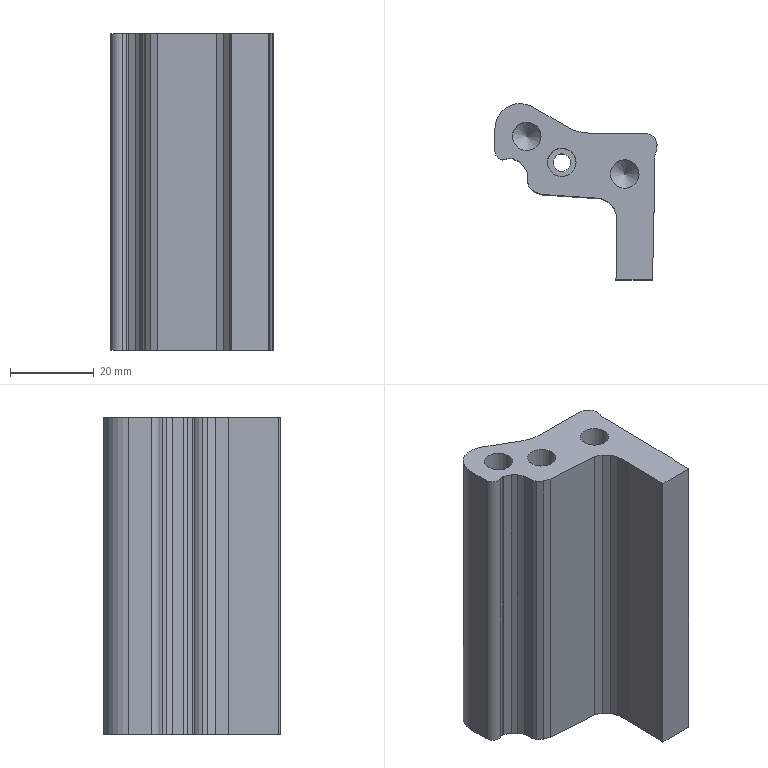Part | NX | features solid 2 | 1 solid | 40 faces | box 38.694 x 42.082 x 75.5 mm | volume 54302 mm3 | plane 26 | cylinder 11 | cone 3 | commonest cylinder face diameters 6.8 x3 4 x2 6 x2 4.2 x1 5.2 x1 12 x1
STEP:
#1=CARTESIAN_POINT('',(63.524,-37.821,-5.5));
#2=VERTEX_POINT('',#1);
#3=CARTESIAN_POINT('',(60.924,-37.821,-5.5));
#4=DIRECTION('',(0.,0.,1.));
#5=DIRECTION('',(1.,0.,0.));
#6=AXIS2_PLACEMENT_3D('',#3,#4,#5);
#7=CIRCLE('',#6,2.6);
#8=EDGE_CURVE('',#2,#2,#7,.T.);
#9=ORIENTED_EDGE('',*,*,#8,.T.);
#10=EDGE_LOOP('',(#9));
#11=FACE_BOUND('',#10,.T.);
#12=CARTESIAN_POINT('',(74.016,-60.221,-5.5));
#13=VERTEX_POINT('',#12);
#14=CARTESIAN_POINT('',(73.954,-65.044,-5.5));
#15=VERTEX_POINT('',#14);
#16=CARTESIAN_POINT('',(74.016,-60.221,-5.5));
#17=DIRECTION('',(-0.01273,-0.9999,0.));
#18=VECTOR('',#17,1000.);
#19=LINE('',#16,#18);
#20=EDGE_CURVE('',#13,#15,#19,.T.);
#21=ORIENTED_EDGE('',*,*,#20,.T.);
#22=CARTESIAN_POINT('',(65.247,-65.044,-5.5));
#23=VERTEX_POINT('',#22);
#24=CARTESIAN_POINT('',(40.003,-65.044,-5.5));
#25=DIRECTION('',(-1.,0.,0.));
#26=VECTOR('',#25,1000.);
#27=LINE('',#24,#26);
#28=EDGE_CURVE('',#15,#23,#27,.T.);
#29=ORIENTED_EDGE('',*,*,#28,.T.);
#30=CARTESIAN_POINT('',(65.303,-64.563,-5.5));
#31=VERTEX_POINT('',#30);
#32=CARTESIAN_POINT('',(63.441,-80.376,-5.5));
#33=DIRECTION('',(0.117,0.9931,0.));
#34=VECTOR('',#33,1000.);
#35=LINE('',#32,#34);
#36=EDGE_CURVE('',#23,#31,#35,.T.);
#37=ORIENTED_EDGE('',*,*,#36,.T.);
#38=CARTESIAN_POINT('',(65.509,-52.772,-5.5));
#39=VERTEX_POINT('',#38);
#40=CARTESIAN_POINT('',(65.303,-64.563,-5.5));
#41=DIRECTION('',(0.01745,0.9998,0.));
#42=VECTOR('',#41,1000.);
#43=LINE('',#40,#42);
#44=EDGE_CURVE('',#31,#39,#43,.T.);
#45=ORIENTED_EDGE('',*,*,#44,.T.);
#46=CARTESIAN_POINT('',(65.447,-49.66,-5.5));
#47=VERTEX_POINT('',#46);
#48=CARTESIAN_POINT('',(65.509,-52.772,-5.5));
#49=DIRECTION('',(-0.02008,0.9998,0.));
#50=VECTOR('',#49,1000.);
#51=LINE('',#48,#50);
#52=EDGE_CURVE('',#39,#47,#51,.T.);
#53=ORIENTED_EDGE('',*,*,#52,.T.);
#54=CARTESIAN_POINT('',(64.727,-47.823,-5.5));
#55=VERTEX_POINT('',#54);
#56=CARTESIAN_POINT('',(65.447,-49.66,-5.5));
#57=DIRECTION('',(-0.3648,0.9311,0.));
#58=VECTOR('',#57,1000.);
#59=LINE('',#56,#58);
#60=EDGE_CURVE('',#47,#55,#59,.T.);
#61=ORIENTED_EDGE('',*,*,#60,.T.);
#62=CARTESIAN_POINT('',(63.388,-46.401,-5.5));
#63=VERTEX_POINT('',#62);
#64=CARTESIAN_POINT('',(64.727,-47.823,-5.5));
#65=DIRECTION('',(-0.6854,0.7281,0.));
#66=VECTOR('',#65,1000.);
#67=LINE('',#64,#66);
#68=EDGE_CURVE('',#55,#63,#67,.T.);
#69=ORIENTED_EDGE('',*,*,#68,.T.);
#70=CARTESIAN_POINT('',(61.633,-45.601,-5.5));
#71=VERTEX_POINT('',#70);
#72=CARTESIAN_POINT('',(63.388,-46.401,-5.5));
#73=DIRECTION('',(-0.9101,0.4145,0.));
#74=VECTOR('',#73,1000.);
#75=LINE('',#72,#74);
#76=EDGE_CURVE('',#63,#71,#75,.T.);
#77=ORIENTED_EDGE('',*,*,#76,.T.);
#78=CARTESIAN_POINT('',(47.584,-44.653,-5.5));
#79=VERTEX_POINT('',#78);
#80=CARTESIAN_POINT('',(61.633,-45.601,-5.5));
#81=DIRECTION('',(-0.9977,0.06737,0.));
#82=VECTOR('',#81,1000.);
#83=LINE('',#80,#82);
#84=EDGE_CURVE('',#71,#79,#83,.T.);
#85=ORIENTED_EDGE('',*,*,#84,.T.);
#86=CARTESIAN_POINT('',(45.844,-44.031,-5.5));
#87=VERTEX_POINT('',#86);
#88=CARTESIAN_POINT('',(47.584,-44.653,-5.5));
#89=DIRECTION('',(-0.9417,0.3365,0.));
#90=VECTOR('',#89,1000.);
#91=LINE('',#88,#90);
#92=EDGE_CURVE('',#79,#87,#91,.T.);
#93=ORIENTED_EDGE('',*,*,#92,.T.);
#94=CARTESIAN_POINT('',(44.613,-42.954,-5.5));
#95=VERTEX_POINT('',#94);
#96=CARTESIAN_POINT('',(45.844,-44.031,-5.5));
#97=DIRECTION('',(-0.7529,0.6581,0.));
#98=VECTOR('',#97,1000.);
#99=LINE('',#96,#98);
#100=EDGE_CURVE('',#87,#95,#99,.T.);
#101=ORIENTED_EDGE('',*,*,#100,.T.);
#102=CARTESIAN_POINT('',(44.296,-42.082,-5.5));
#103=VERTEX_POINT('',#102);
#104=CARTESIAN_POINT('',(44.613,-42.954,-5.5));
#105=DIRECTION('',(-0.3407,0.9402,0.));
#106=VECTOR('',#105,1000.);
#107=LINE('',#104,#106);
#108=EDGE_CURVE('',#95,#103,#107,.T.);
#109=ORIENTED_EDGE('',*,*,#108,.T.);
#110=CARTESIAN_POINT('',(44.079,-39.402,-5.5));
#111=VERTEX_POINT('',#110);
#112=CARTESIAN_POINT('',(44.296,-42.082,-5.5));
#113=DIRECTION('',(-0.08071,0.9967,0.));
#114=VECTOR('',#113,1000.);
#115=LINE('',#112,#114);
#116=EDGE_CURVE('',#103,#111,#115,.T.);
#117=ORIENTED_EDGE('',*,*,#116,.T.);
#118=CARTESIAN_POINT('',(43.3,-37.914,-5.5));
#119=VERTEX_POINT('',#118);
#120=CARTESIAN_POINT('',(44.079,-39.402,-5.5));
#121=DIRECTION('',(-0.4639,0.8859,0.));
#122=VECTOR('',#121,1000.);
#123=LINE('',#120,#122);
#124=EDGE_CURVE('',#111,#119,#123,.T.);
#125=ORIENTED_EDGE('',*,*,#124,.T.);
#126=CARTESIAN_POINT('',(42.234,-36.887,-5.5));
#127=VERTEX_POINT('',#126);
#128=CARTESIAN_POINT('',(43.3,-37.914,-5.5));
#129=DIRECTION('',(-0.7204,0.6936,0.));
#130=VECTOR('',#129,1000.);
#131=LINE('',#128,#130);
#132=EDGE_CURVE('',#119,#127,#131,.T.);
#133=ORIENTED_EDGE('',*,*,#132,.T.);
#134=CARTESIAN_POINT('',(40.597,-36.034,-5.5));
#135=VERTEX_POINT('',#134);
#136=CARTESIAN_POINT('',(42.234,-36.887,-5.5));
#137=DIRECTION('',(-0.8867,0.4624,0.));
#138=VECTOR('',#137,1000.);
#139=LINE('',#136,#138);
#140=EDGE_CURVE('',#127,#135,#139,.T.);
#141=ORIENTED_EDGE('',*,*,#140,.T.);
#142=CARTESIAN_POINT('',(40.213,-35.993,-5.5));
#143=VERTEX_POINT('',#142);
#144=CARTESIAN_POINT('',(40.597,-36.034,-5.5));
#145=DIRECTION('',(-0.9945,0.105,0.));
#146=VECTOR('',#145,1000.);
#147=LINE('',#144,#146);
#148=EDGE_CURVE('',#135,#143,#147,.T.);
#149=ORIENTED_EDGE('',*,*,#148,.T.);
#150=CARTESIAN_POINT('',(39.206,-36.148,-5.5));
#151=VERTEX_POINT('',#150);
#152=CARTESIAN_POINT('',(40.003,-37.982,-5.5));
#153=DIRECTION('',(0.,0.,1.));
#154=DIRECTION('',(1.,0.,0.));
#155=AXIS2_PLACEMENT_3D('',#152,#153,#154);
#156=CIRCLE('',#155,2.);
#157=EDGE_CURVE('',#143,#151,#156,.T.);
#158=ORIENTED_EDGE('',*,*,#157,.T.);
#159=CARTESIAN_POINT('',(36.409,-34.313,-5.5));
#160=VERTEX_POINT('',#159);
#161=CARTESIAN_POINT('',(38.409,-34.313,-5.5));
#162=DIRECTION('',(0.,0.,-1.));
#163=DIRECTION('',(1.,0.,0.));
#164=AXIS2_PLACEMENT_3D('',#161,#162,#163);
#165=CIRCLE('',#164,2.);
#166=EDGE_CURVE('',#151,#160,#165,.T.);
#167=ORIENTED_EDGE('',*,*,#166,.T.);
#168=CARTESIAN_POINT('',(36.409,-28.962,-5.5));
#169=VERTEX_POINT('',#168);
#170=CARTESIAN_POINT('',(36.409,-34.313,-5.5));
#171=DIRECTION('',(0.,1.,0.));
#172=VECTOR('',#171,1000.);
#173=LINE('',#170,#172);
#174=EDGE_CURVE('',#160,#169,#173,.T.);
#175=ORIENTED_EDGE('',*,*,#174,.T.);
#176=CARTESIAN_POINT('',(45.409,-23.765,-5.5));
#177=VERTEX_POINT('',#176);
#178=CARTESIAN_POINT('',(42.409,-28.962,-5.5));
#179=DIRECTION('',(0.,0.,-1.));
#180=DIRECTION('',(1.,0.,0.));
#181=AXIS2_PLACEMENT_3D('',#178,#179,#180);
#182=CIRCLE('',#181,6.);
#183=EDGE_CURVE('',#169,#177,#182,.T.);
#184=ORIENTED_EDGE('',*,*,#183,.T.);
#185=CARTESIAN_POINT('',(53.924,-28.682,-5.5));
#186=VERTEX_POINT('',#185);
#187=CARTESIAN_POINT('',(45.409,-23.765,-5.5));
#188=DIRECTION('',(0.866,-0.5,0.));
#189=VECTOR('',#188,1000.);
#190=LINE('',#187,#189);
#191=EDGE_CURVE('',#177,#186,#190,.T.);
#192=ORIENTED_EDGE('',*,*,#191,.T.);
#193=CARTESIAN_POINT('',(58.924,-30.021,-5.5));
#194=VERTEX_POINT('',#193);
#195=CARTESIAN_POINT('',(58.924,-20.021,-5.5));
#196=DIRECTION('',(0.,0.,1.));
#197=DIRECTION('',(1.,0.,0.));
#198=AXIS2_PLACEMENT_3D('',#195,#196,#197);
#199=CIRCLE('',#198,10.);
#200=EDGE_CURVE('',#186,#194,#199,.T.);
#201=ORIENTED_EDGE('',*,*,#200,.T.);
#202=CARTESIAN_POINT('',(72.102,-30.021,-5.5));
#203=VERTEX_POINT('',#202);
#204=CARTESIAN_POINT('',(58.924,-30.021,-5.5));
#205=DIRECTION('',(1.,0.,0.));
#206=VECTOR('',#205,1000.);
#207=LINE('',#204,#206);
#208=EDGE_CURVE('',#194,#203,#207,.T.);
#209=ORIENTED_EDGE('',*,*,#208,.T.);
#210=CARTESIAN_POINT('',(74.849,-34.228,-5.5));
#211=VERTEX_POINT('',#210);
#212=CARTESIAN_POINT('',(72.102,-33.021,-5.5));
#213=DIRECTION('',(0.,0.,-1.));
#214=DIRECTION('',(1.,0.,0.));
#215=AXIS2_PLACEMENT_3D('',#212,#213,#214);
#216=CIRCLE('',#215,3.);
#217=EDGE_CURVE('',#203,#211,#216,.T.);
#218=ORIENTED_EDGE('',*,*,#217,.T.);
#219=CARTESIAN_POINT('',(74.596,-35.426,-5.5));
#220=VERTEX_POINT('',#219);
#221=CARTESIAN_POINT('',(77.596,-35.434,-5.5));
#222=DIRECTION('',(0.,0.,1.));
#223=DIRECTION('',(1.,0.,0.));
#224=AXIS2_PLACEMENT_3D('',#221,#222,#223);
#225=CIRCLE('',#224,3.);
#226=EDGE_CURVE('',#211,#220,#225,.T.);
#227=ORIENTED_EDGE('',*,*,#226,.T.);
#228=CARTESIAN_POINT('',(74.59,-37.317,-5.5));
#229=VERTEX_POINT('',#228);
#230=CARTESIAN_POINT('',(74.596,-35.426,-5.5));
#231=DIRECTION('',(-0.002751,-1.,0.));
#232=VECTOR('',#231,1000.);
#233=LINE('',#230,#232);
#234=EDGE_CURVE('',#220,#229,#233,.T.);
#235=ORIENTED_EDGE('',*,*,#234,.T.);
#236=CARTESIAN_POINT('',(74.168,-59.593,-5.5));
#237=VERTEX_POINT('',#236);
#238=CARTESIAN_POINT('',(74.59,-37.317,-5.5));
#239=DIRECTION('',(-0.01897,-0.9998,0.));
#240=VECTOR('',#239,1000.);
#241=LINE('',#238,#240);
#242=EDGE_CURVE('',#229,#237,#241,.T.);
#243=ORIENTED_EDGE('',*,*,#242,.T.);
#244=CARTESIAN_POINT('',(74.168,-59.593,-5.5));
#245=DIRECTION('',(-0.2353,-0.9719,0.));
#246=VECTOR('',#245,1000.);
#247=LINE('',#244,#246);
#248=EDGE_CURVE('',#237,#13,#247,.T.);
#249=ORIENTED_EDGE('',*,*,#248,.T.);
#250=EDGE_LOOP('',(#21,#29,#37,#45,#53,#61,#69,#77,#85,#93,#101,#109,#117,#125,#133,#141,#149,#158,#167,#175,#184,#192,#201,#209,#218,#227,#235,#243,#249));
#251=FACE_BOUND('',#250,.T.);
#252=CARTESIAN_POINT('',(54.463,-37.,-5.5));
#253=VERTEX_POINT('',#252);
#254=CARTESIAN_POINT('',(52.363,-37.,-5.5));
#255=DIRECTION('',(0.,0.,1.));
#256=DIRECTION('',(1.,0.,0.));
#257=AXIS2_PLACEMENT_3D('',#254,#255,#256);
#258=CIRCLE('',#257,2.1);
#259=EDGE_CURVE('',#253,#253,#258,.T.);
#260=ORIENTED_EDGE('',*,*,#259,.T.);
#261=EDGE_LOOP('',(#260));
#262=FACE_BOUND('',#261,.T.);
#263=CARTESIAN_POINT('',(40.003,-37.982,-5.5));
#264=DIRECTION('',(0.,0.,1.));
#265=DIRECTION('',(1.,0.,0.));
#266=AXIS2_PLACEMENT_3D('',#263,#264,#265);
#267=PLANE('',#266);
#268=ADVANCED_FACE('',(#11,#251,#262),#267,.F.);
#269=CARTESIAN_POINT('',(70.8,-39.8,70.));
#270=VERTEX_POINT('',#269);
#271=CARTESIAN_POINT('',(67.4,-39.8,70.));
#272=DIRECTION('',(0.,0.,-1.));
#273=DIRECTION('',(1.,0.,0.));
#274=AXIS2_PLACEMENT_3D('',#271,#272,#273);
#275=CIRCLE('',#274,3.4);
#276=EDGE_CURVE('',#270,#270,#275,.T.);
#277=ORIENTED_EDGE('',*,*,#276,.T.);
#278=EDGE_LOOP('',(#277));
#279=FACE_BOUND('',#278,.T.);
#280=CARTESIAN_POINT('',(73.954,-65.044,70.));
#281=VERTEX_POINT('',#280);
#282=CARTESIAN_POINT('',(65.247,-65.044,70.));
#283=VERTEX_POINT('',#282);
#284=CARTESIAN_POINT('',(-37.5,-65.044,70.));
#285=DIRECTION('',(-1.,0.,0.));
#286=VECTOR('',#285,1000.);
#287=LINE('',#284,#286);
#288=EDGE_CURVE('',#281,#283,#287,.T.);
#289=ORIENTED_EDGE('',*,*,#288,.F.);
#290=CARTESIAN_POINT('',(74.016,-60.221,70.));
#291=VERTEX_POINT('',#290);
#292=CARTESIAN_POINT('',(74.016,-60.221,70.));
#293=DIRECTION('',(-0.01273,-0.9999,0.));
#294=VECTOR('',#293,1000.);
#295=LINE('',#292,#294);
#296=EDGE_CURVE('',#291,#281,#295,.T.);
#297=ORIENTED_EDGE('',*,*,#296,.F.);
#298=CARTESIAN_POINT('',(74.168,-59.593,70.));
#299=VERTEX_POINT('',#298);
#300=CARTESIAN_POINT('',(74.168,-59.593,70.));
#301=DIRECTION('',(-0.2353,-0.9719,0.));
#302=VECTOR('',#301,1000.);
#303=LINE('',#300,#302);
#304=EDGE_CURVE('',#299,#291,#303,.T.);
#305=ORIENTED_EDGE('',*,*,#304,.F.);
#306=CARTESIAN_POINT('',(74.59,-37.317,70.));
#307=VERTEX_POINT('',#306);
#308=CARTESIAN_POINT('',(74.59,-37.317,70.));
#309=DIRECTION('',(-0.01897,-0.9998,0.));
#310=VECTOR('',#309,1000.);
#311=LINE('',#308,#310);
#312=EDGE_CURVE('',#307,#299,#311,.T.);
#313=ORIENTED_EDGE('',*,*,#312,.F.);
#314=CARTESIAN_POINT('',(74.596,-35.426,70.));
#315=VERTEX_POINT('',#314);
#316=CARTESIAN_POINT('',(74.596,-35.426,70.));
#317=DIRECTION('',(-0.002751,-1.,0.));
#318=VECTOR('',#317,1000.);
#319=LINE('',#316,#318);
#320=EDGE_CURVE('',#315,#307,#319,.T.);
#321=ORIENTED_EDGE('',*,*,#320,.F.);
#322=CARTESIAN_POINT('',(74.849,-34.228,70.));
#323=VERTEX_POINT('',#322);
#324=CARTESIAN_POINT('',(77.596,-35.434,70.));
#325=DIRECTION('',(0.,0.,1.));
#326=DIRECTION('',(1.,0.,0.));
#327=AXIS2_PLACEMENT_3D('',#324,#325,#326);
#328=CIRCLE('',#327,3.);
#329=EDGE_CURVE('',#323,#315,#328,.T.);
#330=ORIENTED_EDGE('',*,*,#329,.F.);
#331=CARTESIAN_POINT('',(72.102,-30.021,70.));
#332=VERTEX_POINT('',#331);
#333=CARTESIAN_POINT('',(72.102,-33.021,70.));
#334=DIRECTION('',(0.,0.,1.));
#335=DIRECTION('',(1.,0.,0.));
#336=AXIS2_PLACEMENT_3D('',#333,#334,#335);
#337=CIRCLE('',#336,3.);
#338=EDGE_CURVE('',#332,#323,#337,.F.);
#339=ORIENTED_EDGE('',*,*,#338,.F.);
#340=CARTESIAN_POINT('',(58.924,-30.021,70.));
#341=VERTEX_POINT('',#340);
#342=CARTESIAN_POINT('',(58.924,-30.021,70.));
#343=DIRECTION('',(1.,0.,0.));
#344=VECTOR('',#343,1000.);
#345=LINE('',#342,#344);
#346=EDGE_CURVE('',#341,#332,#345,.T.);
#347=ORIENTED_EDGE('',*,*,#346,.F.);
#348=CARTESIAN_POINT('',(53.924,-28.682,70.));
#349=VERTEX_POINT('',#348);
#350=CARTESIAN_POINT('',(58.924,-20.021,70.));
#351=DIRECTION('',(0.,0.,1.));
#352=DIRECTION('',(1.,0.,0.));
#353=AXIS2_PLACEMENT_3D('',#350,#351,#352);
#354=CIRCLE('',#353,10.);
#355=EDGE_CURVE('',#349,#341,#354,.T.);
#356=ORIENTED_EDGE('',*,*,#355,.F.);
#357=CARTESIAN_POINT('',(45.409,-23.765,70.));
#358=VERTEX_POINT('',#357);
#359=CARTESIAN_POINT('',(45.409,-23.765,70.));
#360=DIRECTION('',(0.866,-0.5,0.));
#361=VECTOR('',#360,1000.);
#362=LINE('',#359,#361);
#363=EDGE_CURVE('',#358,#349,#362,.T.);
#364=ORIENTED_EDGE('',*,*,#363,.F.);
#365=CARTESIAN_POINT('',(36.409,-28.962,70.));
#366=VERTEX_POINT('',#365);
#367=CARTESIAN_POINT('',(42.409,-28.962,70.));
#368=DIRECTION('',(0.,0.,1.));
#369=DIRECTION('',(1.,0.,0.));
#370=AXIS2_PLACEMENT_3D('',#367,#368,#369);
#371=CIRCLE('',#370,6.);
#372=EDGE_CURVE('',#366,#358,#371,.F.);
#373=ORIENTED_EDGE('',*,*,#372,.F.);
#374=CARTESIAN_POINT('',(36.409,-34.313,70.));
#375=VERTEX_POINT('',#374);
#376=CARTESIAN_POINT('',(36.409,-34.313,70.));
#377=DIRECTION('',(0.,1.,0.));
#378=VECTOR('',#377,1000.);
#379=LINE('',#376,#378);
#380=EDGE_CURVE('',#375,#366,#379,.T.);
#381=ORIENTED_EDGE('',*,*,#380,.F.);
#382=CARTESIAN_POINT('',(39.206,-36.148,70.));
#383=VERTEX_POINT('',#382);
#384=CARTESIAN_POINT('',(38.409,-34.313,70.));
#385=DIRECTION('',(0.,0.,1.));
#386=DIRECTION('',(1.,0.,0.));
#387=AXIS2_PLACEMENT_3D('',#384,#385,#386);
#388=CIRCLE('',#387,2.);
#389=EDGE_CURVE('',#383,#375,#388,.F.);
#390=ORIENTED_EDGE('',*,*,#389,.F.);
#391=CARTESIAN_POINT('',(40.213,-35.993,70.));
#392=VERTEX_POINT('',#391);
#393=CARTESIAN_POINT('',(40.003,-37.982,70.));
#394=DIRECTION('',(0.,0.,1.));
#395=DIRECTION('',(1.,0.,0.));
#396=AXIS2_PLACEMENT_3D('',#393,#394,#395);
#397=CIRCLE('',#396,2.);
#398=EDGE_CURVE('',#392,#383,#397,.T.);
#399=ORIENTED_EDGE('',*,*,#398,.F.);
#400=CARTESIAN_POINT('',(40.597,-36.034,70.));
#401=VERTEX_POINT('',#400);
#402=CARTESIAN_POINT('',(40.597,-36.034,70.));
#403=DIRECTION('',(-0.9945,0.105,0.));
#404=VECTOR('',#403,1000.);
#405=LINE('',#402,#404);
#406=EDGE_CURVE('',#401,#392,#405,.T.);
#407=ORIENTED_EDGE('',*,*,#406,.F.);
#408=CARTESIAN_POINT('',(42.234,-36.887,70.));
#409=VERTEX_POINT('',#408);
#410=CARTESIAN_POINT('',(42.234,-36.887,70.));
#411=DIRECTION('',(-0.8867,0.4624,0.));
#412=VECTOR('',#411,1000.);
#413=LINE('',#410,#412);
#414=EDGE_CURVE('',#409,#401,#413,.T.);
#415=ORIENTED_EDGE('',*,*,#414,.F.);
#416=CARTESIAN_POINT('',(43.3,-37.914,70.));
#417=VERTEX_POINT('',#416);
#418=CARTESIAN_POINT('',(43.3,-37.914,70.));
#419=DIRECTION('',(-0.7204,0.6936,0.));
#420=VECTOR('',#419,1000.);
#421=LINE('',#418,#420);
#422=EDGE_CURVE('',#417,#409,#421,.T.);
#423=ORIENTED_EDGE('',*,*,#422,.F.);
#424=CARTESIAN_POINT('',(44.079,-39.402,70.));
#425=VERTEX_POINT('',#424);
#426=CARTESIAN_POINT('',(44.079,-39.402,70.));
#427=DIRECTION('',(-0.4639,0.8859,0.));
#428=VECTOR('',#427,1000.);
#429=LINE('',#426,#428);
#430=EDGE_CURVE('',#425,#417,#429,.T.);
#431=ORIENTED_EDGE('',*,*,#430,.F.);
#432=CARTESIAN_POINT('',(44.296,-42.082,70.));
#433=VERTEX_POINT('',#432);
#434=CARTESIAN_POINT('',(44.296,-42.082,70.));
#435=DIRECTION('',(-0.08071,0.9967,0.));
#436=VECTOR('',#435,1000.);
#437=LINE('',#434,#436);
#438=EDGE_CURVE('',#433,#425,#437,.T.);
#439=ORIENTED_EDGE('',*,*,#438,.F.);
#440=CARTESIAN_POINT('',(44.613,-42.954,70.));
#441=VERTEX_POINT('',#440);
#442=CARTESIAN_POINT('',(44.613,-42.954,70.));
#443=DIRECTION('',(-0.3407,0.9402,0.));
#444=VECTOR('',#443,1000.);
#445=LINE('',#442,#444);
#446=EDGE_CURVE('',#441,#433,#445,.T.);
#447=ORIENTED_EDGE('',*,*,#446,.F.);
#448=CARTESIAN_POINT('',(45.844,-44.031,70.));
#449=VERTEX_POINT('',#448);
#450=CARTESIAN_POINT('',(45.844,-44.031,70.));
#451=DIRECTION('',(-0.7529,0.6581,0.));
#452=VECTOR('',#451,1000.);
#453=LINE('',#450,#452);
#454=EDGE_CURVE('',#441,#449,#453,.F.);
#455=ORIENTED_EDGE('',*,*,#454,.T.);
#456=CARTESIAN_POINT('',(47.584,-44.653,70.));
#457=VERTEX_POINT('',#456);
#458=CARTESIAN_POINT('',(47.584,-44.653,70.));
#459=DIRECTION('',(-0.9417,0.3365,0.));
#460=VECTOR('',#459,1000.);
#461=LINE('',#458,#460);
#462=EDGE_CURVE('',#449,#457,#461,.F.);
#463=ORIENTED_EDGE('',*,*,#462,.T.);
#464=CARTESIAN_POINT('',(61.633,-45.601,70.));
#465=VERTEX_POINT('',#464);
#466=CARTESIAN_POINT('',(61.633,-45.601,70.));
#467=DIRECTION('',(-0.9977,0.06737,0.));
#468=VECTOR('',#467,1000.);
#469=LINE('',#466,#468);
#470=EDGE_CURVE('',#457,#465,#469,.F.);
#471=ORIENTED_EDGE('',*,*,#470,.T.);
#472=CARTESIAN_POINT('',(63.388,-46.401,70.));
#473=VERTEX_POINT('',#472);
#474=CARTESIAN_POINT('',(63.388,-46.401,70.));
#475=DIRECTION('',(-0.9101,0.4145,0.));
#476=VECTOR('',#475,1000.);
#477=LINE('',#474,#476);
#478=EDGE_CURVE('',#465,#473,#477,.F.);
#479=ORIENTED_EDGE('',*,*,#478,.T.);
#480=CARTESIAN_POINT('',(64.727,-47.823,70.));
#481=VERTEX_POINT('',#480);
#482=CARTESIAN_POINT('',(64.727,-47.823,70.));
#483=DIRECTION('',(-0.6854,0.7281,0.));
#484=VECTOR('',#483,1000.);
#485=LINE('',#482,#484);
#486=EDGE_CURVE('',#473,#481,#485,.F.);
#487=ORIENTED_EDGE('',*,*,#486,.T.);
#488=CARTESIAN_POINT('',(65.447,-49.66,70.));
#489=VERTEX_POINT('',#488);
#490=CARTESIAN_POINT('',(65.447,-49.66,70.));
#491=DIRECTION('',(-0.3648,0.9311,0.));
#492=VECTOR('',#491,1000.);
#493=LINE('',#490,#492);
#494=EDGE_CURVE('',#481,#489,#493,.F.);
#495=ORIENTED_EDGE('',*,*,#494,.T.);
#496=CARTESIAN_POINT('',(65.509,-52.772,70.));
#497=VERTEX_POINT('',#496);
#498=CARTESIAN_POINT('',(65.509,-52.772,70.));
#499=DIRECTION('',(-0.02008,0.9998,0.));
#500=VECTOR('',#499,1000.);
#501=LINE('',#498,#500);
#502=EDGE_CURVE('',#489,#497,#501,.F.);
#503=ORIENTED_EDGE('',*,*,#502,.T.);
#504=CARTESIAN_POINT('',(65.303,-64.563,70.));
#505=VERTEX_POINT('',#504);
#506=CARTESIAN_POINT('',(65.303,-64.563,70.));
#507=DIRECTION('',(0.01745,0.9998,0.));
#508=VECTOR('',#507,1000.);
#509=LINE('',#506,#508);
#510=EDGE_CURVE('',#497,#505,#509,.F.);
#511=ORIENTED_EDGE('',*,*,#510,.T.);
#512=CARTESIAN_POINT('',(63.441,-80.376,70.));
#513=DIRECTION('',(0.117,0.9931,0.));
#514=VECTOR('',#513,1000.);
#515=LINE('',#512,#514);
#516=EDGE_CURVE('',#505,#283,#515,.F.);
#517=ORIENTED_EDGE('',*,*,#516,.T.);
#518=EDGE_LOOP('',(#289,#297,#305,#313,#321,#330,#339,#347,#356,#364,#373,#381,#390,#399,#407,#415,#423,#431,#439,#447,#455,#463,#471,#479,#487,#495,#503,#511,#517));
#519=FACE_BOUND('',#518,.T.);
#520=CARTESIAN_POINT('',(55.763,-37.,70.));
#521=VERTEX_POINT('',#520);
#522=CARTESIAN_POINT('',(52.363,-37.,70.));
#523=DIRECTION('',(0.,0.,1.));
#524=DIRECTION('',(1.,0.,0.));
#525=AXIS2_PLACEMENT_3D('',#522,#523,#524);
#526=CIRCLE('',#525,3.4);
#527=EDGE_CURVE('',#521,#521,#526,.T.);
#528=ORIENTED_EDGE('',*,*,#527,.F.);
#529=EDGE_LOOP('',(#528));
#530=FACE_BOUND('',#529,.T.);
#531=CARTESIAN_POINT('',(47.4,-30.8,70.));
#532=VERTEX_POINT('',#531);
#533=CARTESIAN_POINT('',(44.,-30.8,70.));
#534=DIRECTION('',(0.,0.,-1.));
#535=DIRECTION('',(1.,0.,0.));
#536=AXIS2_PLACEMENT_3D('',#533,#534,#535);
#537=CIRCLE('',#536,3.4);
#538=EDGE_CURVE('',#532,#532,#537,.T.);
#539=ORIENTED_EDGE('',*,*,#538,.T.);
#540=EDGE_LOOP('',(#539));
#541=FACE_BOUND('',#540,.T.);
#542=CARTESIAN_POINT('',(-37.5,0.,70.));
#543=DIRECTION('',(0.,0.,1.));
#544=DIRECTION('',(1.,0.,0.));
#545=AXIS2_PLACEMENT_3D('',#542,#543,#544);
#546=PLANE('',#545);
#547=ADVANCED_FACE('',(#279,#519,#530,#541),#546,.T.);
#548=ORIENTED_EDGE('',*,*,#510,.F.);
#549=CARTESIAN_POINT('',(65.509,-52.772,40.));
#550=DIRECTION('',(0.,0.,-1.));
#551=VECTOR('',#550,1000.);
#552=LINE('',#549,#551);
#553=EDGE_CURVE('',#497,#39,#552,.T.);
#554=ORIENTED_EDGE('',*,*,#553,.T.);
#555=ORIENTED_EDGE('',*,*,#44,.F.);
#556=CARTESIAN_POINT('',(65.303,-64.563,40.));
#557=DIRECTION('',(0.,0.,-1.));
#558=VECTOR('',#557,1000.);
#559=LINE('',#556,#558);
#560=EDGE_CURVE('',#505,#31,#559,.T.);
#561=ORIENTED_EDGE('',*,*,#560,.F.);
#562=EDGE_LOOP('',(#548,#554,#555,#561));
#563=FACE_BOUND('',#562,.T.);
#564=CARTESIAN_POINT('',(65.303,-64.563,40.));
#565=DIRECTION('',(-0.9998,0.01745,0.));
#566=DIRECTION('',(-0.01745,-0.9998,0.));
#567=AXIS2_PLACEMENT_3D('',#564,#565,#566);
#568=PLANE('',#567);
#569=ADVANCED_FACE('',(#563),#568,.T.);
#570=CARTESIAN_POINT('',(65.247,-65.044,40.));
#571=DIRECTION('',(0.,0.,-1.));
#572=VECTOR('',#571,1000.);
#573=LINE('',#570,#572);
#574=EDGE_CURVE('',#23,#283,#573,.F.);
#575=ORIENTED_EDGE('',*,*,#574,.T.);
#576=ORIENTED_EDGE('',*,*,#516,.F.);
#577=ORIENTED_EDGE('',*,*,#560,.T.);
#578=ORIENTED_EDGE('',*,*,#36,.F.);
#579=EDGE_LOOP('',(#575,#576,#577,#578));
#580=FACE_BOUND('',#579,.T.);
#581=CARTESIAN_POINT('',(63.441,-80.376,40.));
#582=DIRECTION('',(-0.9931,0.117,0.));
#583=DIRECTION('',(-0.117,-0.9931,0.));
#584=AXIS2_PLACEMENT_3D('',#581,#582,#583);
#585=PLANE('',#584);
#586=ADVANCED_FACE('',(#580),#585,.T.);
#587=CARTESIAN_POINT('',(73.954,-65.044,40.));
#588=DIRECTION('',(0.,0.,1.));
#589=VECTOR('',#588,1000.);
#590=LINE('',#587,#589);
#591=EDGE_CURVE('',#15,#281,#590,.T.);
#592=ORIENTED_EDGE('',*,*,#591,.F.);
#593=ORIENTED_EDGE('',*,*,#20,.F.);
#594=CARTESIAN_POINT('',(74.016,-60.221,40.));
#595=DIRECTION('',(0.,0.,-1.));
#596=VECTOR('',#595,1000.);
#597=LINE('',#594,#596);
#598=EDGE_CURVE('',#291,#13,#597,.T.);
#599=ORIENTED_EDGE('',*,*,#598,.F.);
#600=ORIENTED_EDGE('',*,*,#296,.T.);
#601=EDGE_LOOP('',(#592,#593,#599,#600));
#602=FACE_BOUND('',#601,.T.);
#603=CARTESIAN_POINT('',(74.016,-60.221,40.));
#604=DIRECTION('',(0.9999,-0.01273,0.));
#605=DIRECTION('',(0.01273,0.9999,0.));
#606=AXIS2_PLACEMENT_3D('',#603,#604,#605);
#607=PLANE('',#606);
#608=ADVANCED_FACE('',(#602),#607,.T.);
#609=CARTESIAN_POINT('',(74.168,-59.593,40.));
#610=DIRECTION('',(0.,0.,-1.));
#611=VECTOR('',#610,1000.);
#612=LINE('',#609,#611);
#613=EDGE_CURVE('',#299,#237,#612,.T.);
#614=ORIENTED_EDGE('',*,*,#613,.F.);
#615=ORIENTED_EDGE('',*,*,#304,.T.);
#616=ORIENTED_EDGE('',*,*,#598,.T.);
#617=ORIENTED_EDGE('',*,*,#248,.F.);
#618=EDGE_LOOP('',(#614,#615,#616,#617));
#619=FACE_BOUND('',#618,.T.);
#620=CARTESIAN_POINT('',(74.168,-59.593,40.));
#621=DIRECTION('',(0.9719,-0.2353,0.));
#622=DIRECTION('',(0.2353,0.9719,0.));
#623=AXIS2_PLACEMENT_3D('',#620,#621,#622);
#624=PLANE('',#623);
#625=ADVANCED_FACE('',(#619),#624,.T.);
#626=CARTESIAN_POINT('',(74.59,-37.317,40.));
#627=DIRECTION('',(0.,0.,-1.));
#628=VECTOR('',#627,1000.);
#629=LINE('',#626,#628);
#630=EDGE_CURVE('',#307,#229,#629,.T.);
#631=ORIENTED_EDGE('',*,*,#630,.F.);
#632=ORIENTED_EDGE('',*,*,#312,.T.);
#633=ORIENTED_EDGE('',*,*,#613,.T.);
#634=ORIENTED_EDGE('',*,*,#242,.F.);
#635=EDGE_LOOP('',(#631,#632,#633,#634));
#636=FACE_BOUND('',#635,.T.);
#637=CARTESIAN_POINT('',(74.59,-37.317,40.));
#638=DIRECTION('',(0.9998,-0.01897,0.));
#639=DIRECTION('',(0.01897,0.9998,0.));
#640=AXIS2_PLACEMENT_3D('',#637,#638,#639);
#641=PLANE('',#640);
#642=ADVANCED_FACE('',(#636),#641,.T.);
#643=CARTESIAN_POINT('',(74.596,-35.426,40.));
#644=DIRECTION('',(0.,0.,-1.));
#645=VECTOR('',#644,1000.);
#646=LINE('',#643,#645);
#647=EDGE_CURVE('',#315,#220,#646,.T.);
#648=ORIENTED_EDGE('',*,*,#647,.F.);
#649=ORIENTED_EDGE('',*,*,#320,.T.);
#650=ORIENTED_EDGE('',*,*,#630,.T.);
#651=ORIENTED_EDGE('',*,*,#234,.F.);
#652=EDGE_LOOP('',(#648,#649,#650,#651));
#653=FACE_BOUND('',#652,.T.);
#654=CARTESIAN_POINT('',(74.596,-35.426,40.));
#655=DIRECTION('',(1.,-0.002751,0.));
#656=DIRECTION('',(0.002751,1.,0.));
#657=AXIS2_PLACEMENT_3D('',#654,#655,#656);
#658=PLANE('',#657);
#659=ADVANCED_FACE('',(#653),#658,.T.);
#660=CARTESIAN_POINT('',(74.849,-34.228,40.));
#661=DIRECTION('',(0.,0.,-1.));
#662=VECTOR('',#661,1000.);
#663=LINE('',#660,#662);
#664=EDGE_CURVE('',#323,#211,#663,.T.);
#665=ORIENTED_EDGE('',*,*,#664,.F.);
#666=ORIENTED_EDGE('',*,*,#329,.T.);
#667=ORIENTED_EDGE('',*,*,#647,.T.);
#668=ORIENTED_EDGE('',*,*,#226,.F.);
#669=EDGE_LOOP('',(#665,#666,#667,#668));
#670=FACE_BOUND('',#669,.T.);
#671=CARTESIAN_POINT('',(77.596,-35.434,40.));
#672=DIRECTION('',(0.,0.,-1.));
#673=DIRECTION('',(-1.,0.,0.));
#674=AXIS2_PLACEMENT_3D('',#671,#672,#673);
#675=CYLINDRICAL_SURFACE('',#674,3.);
#676=ADVANCED_FACE('',(#670),#675,.F.);
#677=CARTESIAN_POINT('',(72.102,-30.021,40.));
#678=DIRECTION('',(0.,0.,-1.));
#679=VECTOR('',#678,1000.);
#680=LINE('',#677,#679);
#681=EDGE_CURVE('',#332,#203,#680,.T.);
#682=ORIENTED_EDGE('',*,*,#681,.F.);
#683=ORIENTED_EDGE('',*,*,#338,.T.);
#684=ORIENTED_EDGE('',*,*,#664,.T.);
#685=ORIENTED_EDGE('',*,*,#217,.F.);
#686=EDGE_LOOP('',(#682,#683,#684,#685));
#687=FACE_BOUND('',#686,.T.);
#688=CARTESIAN_POINT('',(72.102,-33.021,40.));
#689=DIRECTION('',(0.,0.,-1.));
#690=DIRECTION('',(-1.,0.,0.));
#691=AXIS2_PLACEMENT_3D('',#688,#689,#690);
#692=CYLINDRICAL_SURFACE('',#691,3.);
#693=ADVANCED_FACE('',(#687),#692,.T.);
#694=CARTESIAN_POINT('',(58.924,-30.021,40.));
#695=DIRECTION('',(0.,0.,-1.));
#696=VECTOR('',#695,1000.);
#697=LINE('',#694,#696);
#698=EDGE_CURVE('',#341,#194,#697,.T.);
#699=ORIENTED_EDGE('',*,*,#698,.F.);
#700=ORIENTED_EDGE('',*,*,#346,.T.);
#701=ORIENTED_EDGE('',*,*,#681,.T.);
#702=ORIENTED_EDGE('',*,*,#208,.F.);
#703=EDGE_LOOP('',(#699,#700,#701,#702));
#704=FACE_BOUND('',#703,.T.);
#705=CARTESIAN_POINT('',(58.924,-30.021,40.));
#706=DIRECTION('',(0.,1.,0.));
#707=DIRECTION('',(-1.,0.,0.));
#708=AXIS2_PLACEMENT_3D('',#705,#706,#707);
#709=PLANE('',#708);
#710=ADVANCED_FACE('',(#704),#709,.T.);
#711=CARTESIAN_POINT('',(53.924,-28.682,40.));
#712=DIRECTION('',(0.,0.,-1.));
#713=VECTOR('',#712,1000.);
#714=LINE('',#711,#713);
#715=EDGE_CURVE('',#349,#186,#714,.T.);
#716=ORIENTED_EDGE('',*,*,#715,.F.);
#717=ORIENTED_EDGE('',*,*,#355,.T.);
#718=ORIENTED_EDGE('',*,*,#698,.T.);
#719=ORIENTED_EDGE('',*,*,#200,.F.);
#720=EDGE_LOOP('',(#716,#717,#718,#719));
#721=FACE_BOUND('',#720,.T.);
#722=CARTESIAN_POINT('',(58.924,-20.021,40.));
#723=DIRECTION('',(0.,0.,-1.));
#724=DIRECTION('',(-1.,0.,0.));
#725=AXIS2_PLACEMENT_3D('',#722,#723,#724);
#726=CYLINDRICAL_SURFACE('',#725,10.);
#727=ADVANCED_FACE('',(#721),#726,.F.);
#728=CARTESIAN_POINT('',(45.409,-23.765,40.));
#729=DIRECTION('',(0.,0.,-1.));
#730=VECTOR('',#729,1000.);
#731=LINE('',#728,#730);
#732=EDGE_CURVE('',#358,#177,#731,.T.);
#733=ORIENTED_EDGE('',*,*,#732,.F.);
#734=ORIENTED_EDGE('',*,*,#363,.T.);
#735=ORIENTED_EDGE('',*,*,#715,.T.);
#736=ORIENTED_EDGE('',*,*,#191,.F.);
#737=EDGE_LOOP('',(#733,#734,#735,#736));
#738=FACE_BOUND('',#737,.T.);
#739=CARTESIAN_POINT('',(45.409,-23.765,40.));
#740=DIRECTION('',(0.5,0.866,0.));
#741=DIRECTION('',(-0.866,0.5,0.));
#742=AXIS2_PLACEMENT_3D('',#739,#740,#741);
#743=PLANE('',#742);
#744=ADVANCED_FACE('',(#738),#743,.T.);
#745=CARTESIAN_POINT('',(36.409,-28.962,40.));
#746=DIRECTION('',(0.,0.,-1.));
#747=VECTOR('',#746,1000.);
#748=LINE('',#745,#747);
#749=EDGE_CURVE('',#366,#169,#748,.T.);
#750=ORIENTED_EDGE('',*,*,#749,.F.);
#751=ORIENTED_EDGE('',*,*,#372,.T.);
#752=ORIENTED_EDGE('',*,*,#732,.T.);
#753=ORIENTED_EDGE('',*,*,#183,.F.);
#754=EDGE_LOOP('',(#750,#751,#752,#753));
#755=FACE_BOUND('',#754,.T.);
#756=CARTESIAN_POINT('',(42.409,-28.962,40.));
#757=DIRECTION('',(0.,0.,-1.));
#758=DIRECTION('',(-1.,0.,0.));
#759=AXIS2_PLACEMENT_3D('',#756,#757,#758);
#760=CYLINDRICAL_SURFACE('',#759,6.);
#761=ADVANCED_FACE('',(#755),#760,.T.);
#762=CARTESIAN_POINT('',(36.409,-34.313,40.));
#763=DIRECTION('',(0.,0.,-1.));
#764=VECTOR('',#763,1000.);
#765=LINE('',#762,#764);
#766=EDGE_CURVE('',#375,#160,#765,.T.);
#767=ORIENTED_EDGE('',*,*,#766,.F.);
#768=ORIENTED_EDGE('',*,*,#380,.T.);
#769=ORIENTED_EDGE('',*,*,#749,.T.);
#770=ORIENTED_EDGE('',*,*,#174,.F.);
#771=EDGE_LOOP('',(#767,#768,#769,#770));
#772=FACE_BOUND('',#771,.T.);
#773=CARTESIAN_POINT('',(36.409,-34.313,40.));
#774=DIRECTION('',(-1.,0.,0.));
#775=DIRECTION('',(0.,-1.,0.));
#776=AXIS2_PLACEMENT_3D('',#773,#774,#775);
#777=PLANE('',#776);
#778=ADVANCED_FACE('',(#772),#777,.T.);
#779=CARTESIAN_POINT('',(39.206,-36.148,40.));
#780=DIRECTION('',(0.,0.,-1.));
#781=VECTOR('',#780,1000.);
#782=LINE('',#779,#781);
#783=EDGE_CURVE('',#383,#151,#782,.T.);
#784=ORIENTED_EDGE('',*,*,#783,.F.);
#785=ORIENTED_EDGE('',*,*,#389,.T.);
#786=ORIENTED_EDGE('',*,*,#766,.T.);
#787=ORIENTED_EDGE('',*,*,#166,.F.);
#788=EDGE_LOOP('',(#784,#785,#786,#787));
#789=FACE_BOUND('',#788,.T.);
#790=CARTESIAN_POINT('',(38.409,-34.313,40.));
#791=DIRECTION('',(0.,0.,-1.));
#792=DIRECTION('',(-1.,0.,0.));
#793=AXIS2_PLACEMENT_3D('',#790,#791,#792);
#794=CYLINDRICAL_SURFACE('',#793,2.);
#795=ADVANCED_FACE('',(#789),#794,.T.);
#796=CARTESIAN_POINT('',(40.213,-35.993,40.));
#797=DIRECTION('',(0.,0.,-1.));
#798=VECTOR('',#797,1000.);
#799=LINE('',#796,#798);
#800=EDGE_CURVE('',#392,#143,#799,.T.);
#801=ORIENTED_EDGE('',*,*,#800,.F.);
#802=ORIENTED_EDGE('',*,*,#398,.T.);
#803=ORIENTED_EDGE('',*,*,#783,.T.);
#804=ORIENTED_EDGE('',*,*,#157,.F.);
#805=EDGE_LOOP('',(#801,#802,#803,#804));
#806=FACE_BOUND('',#805,.T.);
#807=CARTESIAN_POINT('',(40.003,-37.982,40.));
#808=DIRECTION('',(0.,0.,-1.));
#809=DIRECTION('',(-1.,0.,0.));
#810=AXIS2_PLACEMENT_3D('',#807,#808,#809);
#811=CYLINDRICAL_SURFACE('',#810,2.);
#812=ADVANCED_FACE('',(#806),#811,.F.);
#813=CARTESIAN_POINT('',(40.597,-36.034,40.));
#814=DIRECTION('',(0.,0.,-1.));
#815=VECTOR('',#814,1000.);
#816=LINE('',#813,#815);
#817=EDGE_CURVE('',#401,#135,#816,.T.);
#818=ORIENTED_EDGE('',*,*,#817,.F.);
#819=ORIENTED_EDGE('',*,*,#406,.T.);
#820=ORIENTED_EDGE('',*,*,#800,.T.);
#821=ORIENTED_EDGE('',*,*,#148,.F.);
#822=EDGE_LOOP('',(#818,#819,#820,#821));
#823=FACE_BOUND('',#822,.T.);
#824=CARTESIAN_POINT('',(40.597,-36.034,40.));
#825=DIRECTION('',(-0.105,-0.9945,0.));
#826=DIRECTION('',(0.9945,-0.105,0.));
#827=AXIS2_PLACEMENT_3D('',#824,#825,#826);
#828=PLANE('',#827);
#829=ADVANCED_FACE('',(#823),#828,.T.);
#830=CARTESIAN_POINT('',(42.234,-36.887,40.));
#831=DIRECTION('',(0.,0.,-1.));
#832=VECTOR('',#831,1000.);
#833=LINE('',#830,#832);
#834=EDGE_CURVE('',#409,#127,#833,.T.);
#835=ORIENTED_EDGE('',*,*,#834,.F.);
#836=ORIENTED_EDGE('',*,*,#414,.T.);
#837=ORIENTED_EDGE('',*,*,#817,.T.);
#838=ORIENTED_EDGE('',*,*,#140,.F.);
#839=EDGE_LOOP('',(#835,#836,#837,#838));
#840=FACE_BOUND('',#839,.T.);
#841=CARTESIAN_POINT('',(42.234,-36.887,40.));
#842=DIRECTION('',(-0.4624,-0.8867,0.));
#843=DIRECTION('',(0.8867,-0.4624,0.));
#844=AXIS2_PLACEMENT_3D('',#841,#842,#843);
#845=PLANE('',#844);
#846=ADVANCED_FACE('',(#840),#845,.T.);
#847=CARTESIAN_POINT('',(43.3,-37.914,40.));
#848=DIRECTION('',(0.,0.,-1.));
#849=VECTOR('',#848,1000.);
#850=LINE('',#847,#849);
#851=EDGE_CURVE('',#417,#119,#850,.T.);
#852=ORIENTED_EDGE('',*,*,#851,.F.);
#853=ORIENTED_EDGE('',*,*,#422,.T.);
#854=ORIENTED_EDGE('',*,*,#834,.T.);
#855=ORIENTED_EDGE('',*,*,#132,.F.);
#856=EDGE_LOOP('',(#852,#853,#854,#855));
#857=FACE_BOUND('',#856,.T.);
#858=CARTESIAN_POINT('',(43.3,-37.914,40.));
#859=DIRECTION('',(-0.6936,-0.7204,0.));
#860=DIRECTION('',(0.7204,-0.6936,0.));
#861=AXIS2_PLACEMENT_3D('',#858,#859,#860);
#862=PLANE('',#861);
#863=ADVANCED_FACE('',(#857),#862,.T.);
#864=CARTESIAN_POINT('',(44.079,-39.402,40.));
#865=DIRECTION('',(0.,0.,-1.));
#866=VECTOR('',#865,1000.);
#867=LINE('',#864,#866);
#868=EDGE_CURVE('',#425,#111,#867,.T.);
#869=ORIENTED_EDGE('',*,*,#868,.F.);
#870=ORIENTED_EDGE('',*,*,#430,.T.);
#871=ORIENTED_EDGE('',*,*,#851,.T.);
#872=ORIENTED_EDGE('',*,*,#124,.F.);
#873=EDGE_LOOP('',(#869,#870,#871,#872));
#874=FACE_BOUND('',#873,.T.);
#875=CARTESIAN_POINT('',(44.079,-39.402,40.));
#876=DIRECTION('',(-0.8859,-0.4639,0.));
#877=DIRECTION('',(0.4639,-0.8859,0.));
#878=AXIS2_PLACEMENT_3D('',#875,#876,#877);
#879=PLANE('',#878);
#880=ADVANCED_FACE('',(#874),#879,.T.);
#881=CARTESIAN_POINT('',(44.296,-42.082,40.));
#882=DIRECTION('',(0.,0.,-1.));
#883=VECTOR('',#882,1000.);
#884=LINE('',#881,#883);
#885=EDGE_CURVE('',#433,#103,#884,.T.);
#886=ORIENTED_EDGE('',*,*,#885,.F.);
#887=ORIENTED_EDGE('',*,*,#438,.T.);
#888=ORIENTED_EDGE('',*,*,#868,.T.);
#889=ORIENTED_EDGE('',*,*,#116,.F.);
#890=EDGE_LOOP('',(#886,#887,#888,#889));
#891=FACE_BOUND('',#890,.T.);
#892=CARTESIAN_POINT('',(44.296,-42.082,40.));
#893=DIRECTION('',(-0.9967,-0.08071,0.));
#894=DIRECTION('',(0.08071,-0.9967,0.));
#895=AXIS2_PLACEMENT_3D('',#892,#893,#894);
#896=PLANE('',#895);
#897=ADVANCED_FACE('',(#891),#896,.T.);
#898=CARTESIAN_POINT('',(44.613,-42.954,40.));
#899=DIRECTION('',(0.,0.,-1.));
#900=VECTOR('',#899,1000.);
#901=LINE('',#898,#900);
#902=EDGE_CURVE('',#441,#95,#901,.T.);
#903=ORIENTED_EDGE('',*,*,#902,.F.);
#904=ORIENTED_EDGE('',*,*,#446,.T.);
#905=ORIENTED_EDGE('',*,*,#885,.T.);
#906=ORIENTED_EDGE('',*,*,#108,.F.);
#907=EDGE_LOOP('',(#903,#904,#905,#906));
#908=FACE_BOUND('',#907,.T.);
#909=CARTESIAN_POINT('',(44.613,-42.954,40.));
#910=DIRECTION('',(-0.9402,-0.3407,0.));
#911=DIRECTION('',(0.3407,-0.9402,0.));
#912=AXIS2_PLACEMENT_3D('',#909,#910,#911);
#913=PLANE('',#912);
#914=ADVANCED_FACE('',(#908),#913,.T.);
#915=ORIENTED_EDGE('',*,*,#454,.F.);
#916=ORIENTED_EDGE('',*,*,#902,.T.);
#917=ORIENTED_EDGE('',*,*,#100,.F.);
#918=CARTESIAN_POINT('',(45.844,-44.031,40.));
#919=DIRECTION('',(0.,0.,-1.));
#920=VECTOR('',#919,1000.);
#921=LINE('',#918,#920);
#922=EDGE_CURVE('',#449,#87,#921,.T.);
#923=ORIENTED_EDGE('',*,*,#922,.F.);
#924=EDGE_LOOP('',(#915,#916,#917,#923));
#925=FACE_BOUND('',#924,.T.);
#926=CARTESIAN_POINT('',(45.844,-44.031,40.));
#927=DIRECTION('',(-0.6581,-0.7529,0.));
#928=DIRECTION('',(0.7529,-0.6581,0.));
#929=AXIS2_PLACEMENT_3D('',#926,#927,#928);
#930=PLANE('',#929);
#931=ADVANCED_FACE('',(#925),#930,.T.);
#932=ORIENTED_EDGE('',*,*,#462,.F.);
#933=ORIENTED_EDGE('',*,*,#922,.T.);
#934=ORIENTED_EDGE('',*,*,#92,.F.);
#935=CARTESIAN_POINT('',(47.584,-44.653,40.));
#936=DIRECTION('',(0.,0.,-1.));
#937=VECTOR('',#936,1000.);
#938=LINE('',#935,#937);
#939=EDGE_CURVE('',#457,#79,#938,.T.);
#940=ORIENTED_EDGE('',*,*,#939,.F.);
#941=EDGE_LOOP('',(#932,#933,#934,#940));
#942=FACE_BOUND('',#941,.T.);
#943=CARTESIAN_POINT('',(47.584,-44.653,40.));
#944=DIRECTION('',(-0.3365,-0.9417,0.));
#945=DIRECTION('',(0.9417,-0.3365,0.));
#946=AXIS2_PLACEMENT_3D('',#943,#944,#945);
#947=PLANE('',#946);
#948=ADVANCED_FACE('',(#942),#947,.T.);
#949=ORIENTED_EDGE('',*,*,#470,.F.);
#950=ORIENTED_EDGE('',*,*,#939,.T.);
#951=ORIENTED_EDGE('',*,*,#84,.F.);
#952=CARTESIAN_POINT('',(61.633,-45.601,40.));
#953=DIRECTION('',(0.,0.,-1.));
#954=VECTOR('',#953,1000.);
#955=LINE('',#952,#954);
#956=EDGE_CURVE('',#465,#71,#955,.T.);
#957=ORIENTED_EDGE('',*,*,#956,.F.);
#958=EDGE_LOOP('',(#949,#950,#951,#957));
#959=FACE_BOUND('',#958,.T.);
#960=CARTESIAN_POINT('',(61.633,-45.601,40.));
#961=DIRECTION('',(-0.06737,-0.9977,0.));
#962=DIRECTION('',(0.9977,-0.06737,0.));
#963=AXIS2_PLACEMENT_3D('',#960,#961,#962);
#964=PLANE('',#963);
#965=ADVANCED_FACE('',(#959),#964,.T.);
#966=ORIENTED_EDGE('',*,*,#478,.F.);
#967=ORIENTED_EDGE('',*,*,#956,.T.);
#968=ORIENTED_EDGE('',*,*,#76,.F.);
#969=CARTESIAN_POINT('',(63.388,-46.401,40.));
#970=DIRECTION('',(0.,0.,-1.));
#971=VECTOR('',#970,1000.);
#972=LINE('',#969,#971);
#973=EDGE_CURVE('',#473,#63,#972,.T.);
#974=ORIENTED_EDGE('',*,*,#973,.F.);
#975=EDGE_LOOP('',(#966,#967,#968,#974));
#976=FACE_BOUND('',#975,.T.);
#977=CARTESIAN_POINT('',(63.388,-46.401,40.));
#978=DIRECTION('',(-0.4145,-0.9101,0.));
#979=DIRECTION('',(0.9101,-0.4145,0.));
#980=AXIS2_PLACEMENT_3D('',#977,#978,#979);
#981=PLANE('',#980);
#982=ADVANCED_FACE('',(#976),#981,.T.);
#983=ORIENTED_EDGE('',*,*,#486,.F.);
#984=ORIENTED_EDGE('',*,*,#973,.T.);
#985=ORIENTED_EDGE('',*,*,#68,.F.);
#986=CARTESIAN_POINT('',(64.727,-47.823,40.));
#987=DIRECTION('',(0.,0.,-1.));
#988=VECTOR('',#987,1000.);
#989=LINE('',#986,#988);
#990=EDGE_CURVE('',#481,#55,#989,.T.);
#991=ORIENTED_EDGE('',*,*,#990,.F.);
#992=EDGE_LOOP('',(#983,#984,#985,#991));
#993=FACE_BOUND('',#992,.T.);
#994=CARTESIAN_POINT('',(64.727,-47.823,40.));
#995=DIRECTION('',(-0.7281,-0.6854,0.));
#996=DIRECTION('',(0.6854,-0.7281,0.));
#997=AXIS2_PLACEMENT_3D('',#994,#995,#996);
#998=PLANE('',#997);
#999=ADVANCED_FACE('',(#993),#998,.T.);
#1000=ORIENTED_EDGE('',*,*,#494,.F.);
#1001=ORIENTED_EDGE('',*,*,#990,.T.);
#1002=ORIENTED_EDGE('',*,*,#60,.F.);
#1003=CARTESIAN_POINT('',(65.447,-49.66,40.));
#1004=DIRECTION('',(0.,0.,-1.));
#1005=VECTOR('',#1004,1000.);
#1006=LINE('',#1003,#1005);
#1007=EDGE_CURVE('',#489,#47,#1006,.T.);
#1008=ORIENTED_EDGE('',*,*,#1007,.F.);
#1009=EDGE_LOOP('',(#1000,#1001,#1002,#1008));
#1010=FACE_BOUND('',#1009,.T.);
#1011=CARTESIAN_POINT('',(65.447,-49.66,40.));
#1012=DIRECTION('',(-0.9311,-0.3648,0.));
#1013=DIRECTION('',(0.3648,-0.9311,0.));
#1014=AXIS2_PLACEMENT_3D('',#1011,#1012,#1013);
#1015=PLANE('',#1014);
#1016=ADVANCED_FACE('',(#1010),#1015,.T.);
#1017=ORIENTED_EDGE('',*,*,#502,.F.);
#1018=ORIENTED_EDGE('',*,*,#1007,.T.);
#1019=ORIENTED_EDGE('',*,*,#52,.F.);
#1020=ORIENTED_EDGE('',*,*,#553,.F.);
#1021=EDGE_LOOP('',(#1017,#1018,#1019,#1020));
#1022=FACE_BOUND('',#1021,.T.);
#1023=CARTESIAN_POINT('',(65.509,-52.772,40.));
#1024=DIRECTION('',(-0.9998,-0.02008,0.));
#1025=DIRECTION('',(0.02008,-0.9998,0.));
#1026=AXIS2_PLACEMENT_3D('',#1023,#1024,#1025);
#1027=PLANE('',#1026);
#1028=ADVANCED_FACE('',(#1022),#1027,.T.);
#1029=CARTESIAN_POINT('',(50.263,-37.,29.5));
#1030=VERTEX_POINT('',#1029);
#1031=CARTESIAN_POINT('',(52.363,-37.,29.5));
#1032=DIRECTION('',(0.,0.,-1.));
#1033=DIRECTION('',(-1.,0.,0.));
#1034=AXIS2_PLACEMENT_3D('',#1031,#1032,#1033);
#1035=CIRCLE('',#1034,2.1);
#1036=EDGE_CURVE('',#1030,#1030,#1035,.T.);
#1037=ORIENTED_EDGE('',*,*,#1036,.F.);
#1038=EDGE_LOOP('',(#1037));
#1039=FACE_BOUND('',#1038,.T.);
#1040=ORIENTED_EDGE('',*,*,#259,.F.);
#1041=EDGE_LOOP('',(#1040));
#1042=FACE_BOUND('',#1041,.T.);
#1043=CARTESIAN_POINT('',(52.363,-37.,32.5));
#1044=DIRECTION('',(0.,0.,-1.));
#1045=DIRECTION('',(1.,0.,0.));
#1046=AXIS2_PLACEMENT_3D('',#1043,#1044,#1045);
#1047=CYLINDRICAL_SURFACE('',#1046,2.1);
#1048=ADVANCED_FACE('',(#1039,#1042),#1047,.F.);
#1049=ORIENTED_EDGE('',*,*,#1036,.T.);
#1050=EDGE_LOOP('',(#1049));
#1051=FACE_BOUND('',#1050,.T.);
#1052=CARTESIAN_POINT('',(55.763,-37.,29.5));
#1053=VERTEX_POINT('',#1052);
#1054=CARTESIAN_POINT('',(52.363,-37.,29.5));
#1055=DIRECTION('',(0.,0.,1.));
#1056=DIRECTION('',(1.,0.,0.));
#1057=AXIS2_PLACEMENT_3D('',#1054,#1055,#1056);
#1058=CIRCLE('',#1057,3.4);
#1059=EDGE_CURVE('',#1053,#1053,#1058,.F.);
#1060=ORIENTED_EDGE('',*,*,#1059,.F.);
#1061=EDGE_LOOP('',(#1060));
#1062=FACE_BOUND('',#1061,.T.);
#1063=CARTESIAN_POINT('',(52.363,-37.,29.5));
#1064=DIRECTION('',(0.,0.,-1.));
#1065=DIRECTION('',(-1.,0.,0.));
#1066=AXIS2_PLACEMENT_3D('',#1063,#1064,#1065);
#1067=PLANE('',#1066);
#1068=ADVANCED_FACE('',(#1051,#1062),#1067,.F.);
#1069=ORIENTED_EDGE('',*,*,#527,.T.);
#1070=EDGE_LOOP('',(#1069));
#1071=FACE_BOUND('',#1070,.T.);
#1072=ORIENTED_EDGE('',*,*,#1059,.T.);
#1073=EDGE_LOOP('',(#1072));
#1074=FACE_BOUND('',#1073,.T.);
#1075=CARTESIAN_POINT('',(52.363,-37.,29.5));
#1076=DIRECTION('',(0.,0.,1.));
#1077=DIRECTION('',(1.,0.,0.));
#1078=AXIS2_PLACEMENT_3D('',#1075,#1076,#1077);
#1079=CYLINDRICAL_SURFACE('',#1078,3.4);
#1080=ADVANCED_FACE('',(#1071,#1074),#1079,.F.);
#1081=ORIENTED_EDGE('',*,*,#591,.T.);
#1082=ORIENTED_EDGE('',*,*,#288,.T.);
#1083=ORIENTED_EDGE('',*,*,#574,.F.);
#1084=ORIENTED_EDGE('',*,*,#28,.F.);
#1085=EDGE_LOOP('',(#1081,#1082,#1083,#1084));
#1086=FACE_BOUND('',#1085,.T.);
#1087=CARTESIAN_POINT('',(11.506,-65.044,0.));
#1088=DIRECTION('',(0.,1.,0.));
#1089=DIRECTION('',(0.,0.,1.));
#1090=AXIS2_PLACEMENT_3D('',#1087,#1088,#1089);
#1091=PLANE('',#1090);
#1092=ADVANCED_FACE('',(#1086),#1091,.F.);
#1093=CARTESIAN_POINT('',(64.,-39.8,44.4));
#1094=VERTEX_POINT('',#1093);
#1095=CARTESIAN_POINT('',(67.4,-39.8,44.4));
#1096=DIRECTION('',(0.,0.,-1.));
#1097=DIRECTION('',(-1.,0.,0.));
#1098=AXIS2_PLACEMENT_3D('',#1095,#1096,#1097);
#1099=CIRCLE('',#1098,3.4);
#1100=EDGE_CURVE('',#1094,#1094,#1099,.T.);
#1101=ORIENTED_EDGE('',*,*,#1100,.T.);
#1102=EDGE_LOOP('',(#1101));
#1103=FACE_BOUND('',#1102,.T.);
#1104=ORIENTED_EDGE('',*,*,#276,.F.);
#1105=EDGE_LOOP('',(#1104));
#1106=FACE_BOUND('',#1105,.T.);
#1107=CARTESIAN_POINT('',(67.4,-39.8,70.));
#1108=DIRECTION('',(0.,0.,-1.));
#1109=DIRECTION('',(1.,0.,0.));
#1110=AXIS2_PLACEMENT_3D('',#1107,#1108,#1109);
#1111=CYLINDRICAL_SURFACE('',#1110,3.4);
#1112=ADVANCED_FACE('',(#1103,#1106),#1111,.F.);
#1113=CARTESIAN_POINT('',(67.4,-39.8,41.));
#1114=VERTEX_POINT('',#1113);
#1115=VERTEX_LOOP('',#1114);
#1116=FACE_BOUND('',#1115,.T.);
#1117=ORIENTED_EDGE('',*,*,#1100,.F.);
#1118=EDGE_LOOP('',(#1117));
#1119=FACE_BOUND('',#1118,.T.);
#1120=CARTESIAN_POINT('',(67.4,-39.8,44.4));
#1121=DIRECTION('',(0.,0.,1.));
#1122=DIRECTION('',(1.,0.,0.));
#1123=AXIS2_PLACEMENT_3D('',#1120,#1121,#1122);
#1124=CONICAL_SURFACE('',#1123,3.4,0.7854);
#1125=ADVANCED_FACE('',(#1116,#1119),#1124,.F.);
#1126=CARTESIAN_POINT('',(40.6,-30.8,44.4));
#1127=VERTEX_POINT('',#1126);
#1128=CARTESIAN_POINT('',(44.,-30.8,44.4));
#1129=DIRECTION('',(0.,0.,-1.));
#1130=DIRECTION('',(-1.,0.,0.));
#1131=AXIS2_PLACEMENT_3D('',#1128,#1129,#1130);
#1132=CIRCLE('',#1131,3.4);
#1133=EDGE_CURVE('',#1127,#1127,#1132,.T.);
#1134=ORIENTED_EDGE('',*,*,#1133,.T.);
#1135=EDGE_LOOP('',(#1134));
#1136=FACE_BOUND('',#1135,.T.);
#1137=ORIENTED_EDGE('',*,*,#538,.F.);
#1138=EDGE_LOOP('',(#1137));
#1139=FACE_BOUND('',#1138,.T.);
#1140=CARTESIAN_POINT('',(44.,-30.8,70.));
#1141=DIRECTION('',(0.,0.,-1.));
#1142=DIRECTION('',(1.,0.,0.));
#1143=AXIS2_PLACEMENT_3D('',#1140,#1141,#1142);
#1144=CYLINDRICAL_SURFACE('',#1143,3.4);
#1145=ADVANCED_FACE('',(#1136,#1139),#1144,.F.);
#1146=CARTESIAN_POINT('',(44.,-30.8,41.));
#1147=VERTEX_POINT('',#1146);
#1148=VERTEX_LOOP('',#1147);
#1149=FACE_BOUND('',#1148,.T.);
#1150=ORIENTED_EDGE('',*,*,#1133,.F.);
#1151=EDGE_LOOP('',(#1150));
#1152=FACE_BOUND('',#1151,.T.);
#1153=CARTESIAN_POINT('',(44.,-30.8,44.4));
#1154=DIRECTION('',(0.,0.,1.));
#1155=DIRECTION('',(1.,0.,0.));
#1156=AXIS2_PLACEMENT_3D('',#1153,#1154,#1155);
#1157=CONICAL_SURFACE('',#1156,3.4,0.7854);
#1158=ADVANCED_FACE('',(#1149,#1152),#1157,.F.);
#1159=CARTESIAN_POINT('',(58.324,-37.821,15.9));
#1160=VERTEX_POINT('',#1159);
#1161=CARTESIAN_POINT('',(60.924,-37.821,15.9));
#1162=DIRECTION('',(0.,0.,-1.));
#1163=DIRECTION('',(-1.,0.,0.));
#1164=AXIS2_PLACEMENT_3D('',#1161,#1162,#1163);
#1165=CIRCLE('',#1164,2.6);
#1166=EDGE_CURVE('',#1160,#1160,#1165,.F.);
#1167=ORIENTED_EDGE('',*,*,#1166,.T.);
#1168=EDGE_LOOP('',(#1167));
#1169=FACE_BOUND('',#1168,.T.);
#1170=ORIENTED_EDGE('',*,*,#8,.F.);
#1171=EDGE_LOOP('',(#1170));
#1172=FACE_BOUND('',#1171,.T.);
#1173=CARTESIAN_POINT('',(60.924,-37.821,-5.5));
#1174=DIRECTION('',(0.,0.,1.));
#1175=DIRECTION('',(1.,0.,0.));
#1176=AXIS2_PLACEMENT_3D('',#1173,#1174,#1175);
#1177=CYLINDRICAL_SURFACE('',#1176,2.6);
#1178=ADVANCED_FACE('',(#1169,#1172),#1177,.F.);
#1179=CARTESIAN_POINT('',(60.924,-37.821,18.5));
#1180=VERTEX_POINT('',#1179);
#1181=VERTEX_LOOP('',#1180);
#1182=FACE_BOUND('',#1181,.T.);
#1183=ORIENTED_EDGE('',*,*,#1166,.F.);
#1184=EDGE_LOOP('',(#1183));
#1185=FACE_BOUND('',#1184,.T.);
#1186=CARTESIAN_POINT('',(60.924,-37.821,15.9));
#1187=DIRECTION('',(0.,0.,-1.));
#1188=DIRECTION('',(-1.,0.,0.));
#1189=AXIS2_PLACEMENT_3D('',#1186,#1187,#1188);
#1190=CONICAL_SURFACE('',#1189,2.599,0.7854);
#1191=ADVANCED_FACE('',(#1182,#1185),#1190,.F.);
#1192=CLOSED_SHELL('',(#268,#547,#569,#586,#608,#625,#642,#659,#676,#693,#710,#727,#744,#761,#778,#795,#812,#829,#846,#863,#880,#897,#914,#931,#948,#965,#982,#999,#1016,#1028,#1048,#1068,#1080,#1092,#1112,#1125,#1145,#1158,#1178,#1191));
#1193=MANIFOLD_SOLID_BREP('',#1192);
#1194=(LENGTH_UNIT()NAMED_UNIT(*)SI_UNIT(.MILLI.,.METRE.));
#1195=UNCERTAINTY_MEASURE_WITH_UNIT(LENGTH_MEASURE(0.00001),#1194,'','');
#1196=(NAMED_UNIT(*)PLANE_ANGLE_UNIT()SI_UNIT($,.RADIAN.));
#1197=(NAMED_UNIT(*)SI_UNIT($,.STERADIAN.)SOLID_ANGLE_UNIT());
#1198=(GEOMETRIC_REPRESENTATION_CONTEXT(3)GLOBAL_UNCERTAINTY_ASSIGNED_CONTEXT((#1195))GLOBAL_UNIT_ASSIGNED_CONTEXT((#1194,#1196,#1197))REPRESENTATION_CONTEXT('',''));
#1199=ADVANCED_BREP_SHAPE_REPRESENTATION('',(#1193),#1198);